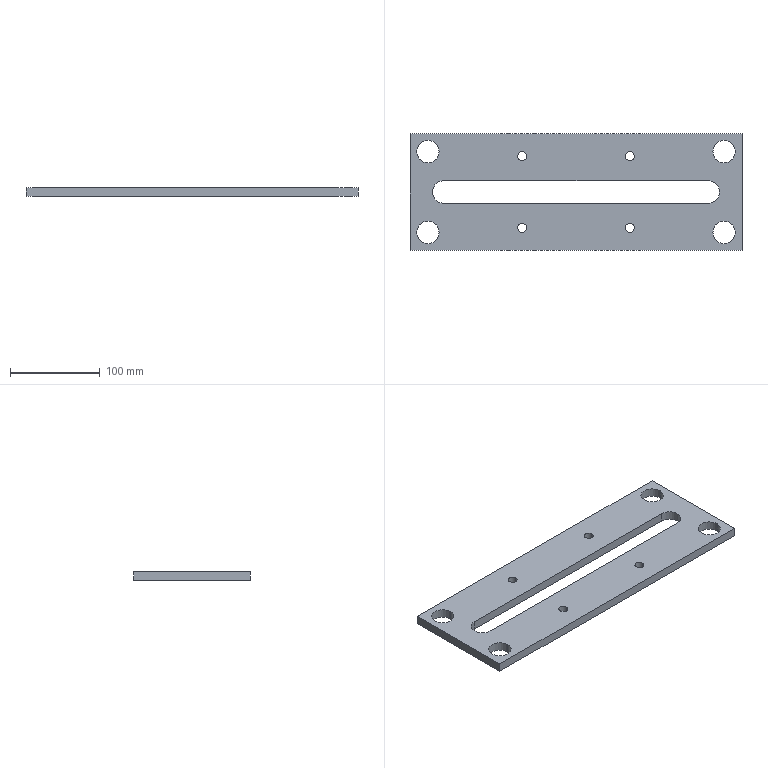Part | SolidWorks | features Extrusion 1, HoleWzd 1 | 1 solid | 27 faces | box 370 x 130 x 10 mm | volume 379565 mm3 | cylinder 19 | plane 8 | commonest cylinder face diameters 25 x11 10 x8
STEP:
#1=CARTESIAN_POINT('',(250.,25.,10.));
#2=VERTEX_POINT('',#1);
#3=CARTESIAN_POINT('',(240.,25.,10.));
#4=VERTEX_POINT('',#3);
#5=CARTESIAN_POINT('',(245.,25.,10.));
#6=DIRECTION('',(0.,0.,-1.));
#7=DIRECTION('',(-1.,0.,0.));
#8=AXIS2_PLACEMENT_3D('',#5,#6,#7);
#9=CIRCLE('',#8,5.);
#10=EDGE_CURVE('',#2,#4,#9,.T.);
#11=ORIENTED_EDGE('',*,*,#10,.F.);
#12=CARTESIAN_POINT('',(250.,25.,0.));
#13=VERTEX_POINT('',#12);
#14=CARTESIAN_POINT('',(250.,25.,0.));
#15=DIRECTION('',(0.,0.,-1.));
#16=VECTOR('',#15,1000.);
#17=LINE('',#14,#16);
#18=EDGE_CURVE('',#2,#13,#17,.T.);
#19=ORIENTED_EDGE('',*,*,#18,.T.);
#20=CARTESIAN_POINT('',(240.,25.,0.));
#21=VERTEX_POINT('',#20);
#22=CARTESIAN_POINT('',(245.,25.,0.));
#23=DIRECTION('',(0.,0.,-1.));
#24=DIRECTION('',(-1.,0.,0.));
#25=AXIS2_PLACEMENT_3D('',#22,#23,#24);
#26=CIRCLE('',#25,5.);
#27=EDGE_CURVE('',#13,#21,#26,.T.);
#28=ORIENTED_EDGE('',*,*,#27,.T.);
#29=CARTESIAN_POINT('',(240.,25.,0.));
#30=DIRECTION('',(0.,0.,-1.));
#31=VECTOR('',#30,1000.);
#32=LINE('',#29,#31);
#33=EDGE_CURVE('',#4,#21,#32,.T.);
#34=ORIENTED_EDGE('',*,*,#33,.F.);
#35=EDGE_LOOP('',(#11,#19,#28,#34));
#36=FACE_OUTER_BOUND('',#35,.T.);
#37=CARTESIAN_POINT('',(245.,25.,0.));
#38=DIRECTION('',(0.,0.,-1.));
#39=DIRECTION('',(-1.,0.,0.));
#40=AXIS2_PLACEMENT_3D('',#37,#38,#39);
#41=CYLINDRICAL_SURFACE('',#40,5.);
#42=ADVANCED_FACE('',(#36),#41,.F.);
#43=CARTESIAN_POINT('',(130.,25.,10.));
#44=VERTEX_POINT('',#43);
#45=CARTESIAN_POINT('',(120.,25.,10.));
#46=VERTEX_POINT('',#45);
#47=CARTESIAN_POINT('',(125.,25.,10.));
#48=DIRECTION('',(0.,0.,-1.));
#49=DIRECTION('',(-1.,0.,0.));
#50=AXIS2_PLACEMENT_3D('',#47,#48,#49);
#51=CIRCLE('',#50,5.);
#52=EDGE_CURVE('',#44,#46,#51,.T.);
#53=ORIENTED_EDGE('',*,*,#52,.F.);
#54=CARTESIAN_POINT('',(130.,25.,0.));
#55=VERTEX_POINT('',#54);
#56=CARTESIAN_POINT('',(130.,25.,0.));
#57=DIRECTION('',(0.,0.,-1.));
#58=VECTOR('',#57,1000.);
#59=LINE('',#56,#58);
#60=EDGE_CURVE('',#44,#55,#59,.T.);
#61=ORIENTED_EDGE('',*,*,#60,.T.);
#62=CARTESIAN_POINT('',(120.,25.,0.));
#63=VERTEX_POINT('',#62);
#64=CARTESIAN_POINT('',(125.,25.,0.));
#65=DIRECTION('',(0.,0.,-1.));
#66=DIRECTION('',(-1.,0.,0.));
#67=AXIS2_PLACEMENT_3D('',#64,#65,#66);
#68=CIRCLE('',#67,5.);
#69=EDGE_CURVE('',#55,#63,#68,.T.);
#70=ORIENTED_EDGE('',*,*,#69,.T.);
#71=CARTESIAN_POINT('',(120.,25.,0.));
#72=DIRECTION('',(0.,0.,-1.));
#73=VECTOR('',#72,1000.);
#74=LINE('',#71,#73);
#75=EDGE_CURVE('',#46,#63,#74,.T.);
#76=ORIENTED_EDGE('',*,*,#75,.F.);
#77=EDGE_LOOP('',(#53,#61,#70,#76));
#78=FACE_OUTER_BOUND('',#77,.T.);
#79=CARTESIAN_POINT('',(125.,25.,0.));
#80=DIRECTION('',(0.,0.,-1.));
#81=DIRECTION('',(-1.,0.,0.));
#82=AXIS2_PLACEMENT_3D('',#79,#80,#81);
#83=CYLINDRICAL_SURFACE('',#82,5.);
#84=ADVANCED_FACE('',(#78),#83,.F.);
#85=CARTESIAN_POINT('',(130.,105.,10.));
#86=VERTEX_POINT('',#85);
#87=CARTESIAN_POINT('',(120.,105.,10.));
#88=VERTEX_POINT('',#87);
#89=CARTESIAN_POINT('',(125.,105.,10.));
#90=DIRECTION('',(0.,0.,-1.));
#91=DIRECTION('',(-1.,0.,0.));
#92=AXIS2_PLACEMENT_3D('',#89,#90,#91);
#93=CIRCLE('',#92,5.);
#94=EDGE_CURVE('',#86,#88,#93,.T.);
#95=ORIENTED_EDGE('',*,*,#94,.F.);
#96=CARTESIAN_POINT('',(130.,105.,0.));
#97=VERTEX_POINT('',#96);
#98=CARTESIAN_POINT('',(130.,105.,0.));
#99=DIRECTION('',(0.,0.,-1.));
#100=VECTOR('',#99,1000.);
#101=LINE('',#98,#100);
#102=EDGE_CURVE('',#86,#97,#101,.T.);
#103=ORIENTED_EDGE('',*,*,#102,.T.);
#104=CARTESIAN_POINT('',(120.,105.,0.));
#105=VERTEX_POINT('',#104);
#106=CARTESIAN_POINT('',(125.,105.,0.));
#107=DIRECTION('',(0.,0.,-1.));
#108=DIRECTION('',(-1.,0.,0.));
#109=AXIS2_PLACEMENT_3D('',#106,#107,#108);
#110=CIRCLE('',#109,5.);
#111=EDGE_CURVE('',#97,#105,#110,.T.);
#112=ORIENTED_EDGE('',*,*,#111,.T.);
#113=CARTESIAN_POINT('',(120.,105.,0.));
#114=DIRECTION('',(0.,0.,-1.));
#115=VECTOR('',#114,1000.);
#116=LINE('',#113,#115);
#117=EDGE_CURVE('',#88,#105,#116,.T.);
#118=ORIENTED_EDGE('',*,*,#117,.F.);
#119=EDGE_LOOP('',(#95,#103,#112,#118));
#120=FACE_OUTER_BOUND('',#119,.T.);
#121=CARTESIAN_POINT('',(125.,105.,0.));
#122=DIRECTION('',(0.,0.,-1.));
#123=DIRECTION('',(-1.,0.,0.));
#124=AXIS2_PLACEMENT_3D('',#121,#122,#123);
#125=CYLINDRICAL_SURFACE('',#124,5.);
#126=ADVANCED_FACE('',(#120),#125,.F.);
#127=CARTESIAN_POINT('',(250.,105.,10.));
#128=VERTEX_POINT('',#127);
#129=CARTESIAN_POINT('',(240.,105.,10.));
#130=VERTEX_POINT('',#129);
#131=CARTESIAN_POINT('',(245.,105.,10.));
#132=DIRECTION('',(0.,0.,-1.));
#133=DIRECTION('',(-1.,0.,0.));
#134=AXIS2_PLACEMENT_3D('',#131,#132,#133);
#135=CIRCLE('',#134,5.);
#136=EDGE_CURVE('',#128,#130,#135,.T.);
#137=ORIENTED_EDGE('',*,*,#136,.F.);
#138=CARTESIAN_POINT('',(250.,105.,0.));
#139=VERTEX_POINT('',#138);
#140=CARTESIAN_POINT('',(250.,105.,0.));
#141=DIRECTION('',(0.,0.,-1.));
#142=VECTOR('',#141,1000.);
#143=LINE('',#140,#142);
#144=EDGE_CURVE('',#128,#139,#143,.T.);
#145=ORIENTED_EDGE('',*,*,#144,.T.);
#146=CARTESIAN_POINT('',(240.,105.,0.));
#147=VERTEX_POINT('',#146);
#148=CARTESIAN_POINT('',(245.,105.,0.));
#149=DIRECTION('',(0.,0.,-1.));
#150=DIRECTION('',(-1.,0.,0.));
#151=AXIS2_PLACEMENT_3D('',#148,#149,#150);
#152=CIRCLE('',#151,5.);
#153=EDGE_CURVE('',#139,#147,#152,.T.);
#154=ORIENTED_EDGE('',*,*,#153,.T.);
#155=CARTESIAN_POINT('',(240.,105.,0.));
#156=DIRECTION('',(0.,0.,-1.));
#157=VECTOR('',#156,1000.);
#158=LINE('',#155,#157);
#159=EDGE_CURVE('',#130,#147,#158,.T.);
#160=ORIENTED_EDGE('',*,*,#159,.F.);
#161=EDGE_LOOP('',(#137,#145,#154,#160));
#162=FACE_OUTER_BOUND('',#161,.T.);
#163=CARTESIAN_POINT('',(245.,105.,0.));
#164=DIRECTION('',(0.,0.,-1.));
#165=DIRECTION('',(-1.,0.,0.));
#166=AXIS2_PLACEMENT_3D('',#163,#164,#165);
#167=CYLINDRICAL_SURFACE('',#166,5.);
#168=ADVANCED_FACE('',(#162),#167,.F.);
#169=CARTESIAN_POINT('',(32.5,20.,10.));
#170=VERTEX_POINT('',#169);
#171=CARTESIAN_POINT('',(7.5,20.,10.));
#172=VERTEX_POINT('',#171);
#173=CARTESIAN_POINT('',(20.,20.,10.));
#174=DIRECTION('',(0.,0.,-1.));
#175=DIRECTION('',(1.,0.,0.));
#176=AXIS2_PLACEMENT_3D('',#173,#174,#175);
#177=CIRCLE('',#176,12.5);
#178=EDGE_CURVE('',#170,#172,#177,.T.);
#179=ORIENTED_EDGE('',*,*,#178,.F.);
#180=CARTESIAN_POINT('',(32.5,20.,0.));
#181=VERTEX_POINT('',#180);
#182=CARTESIAN_POINT('',(32.5,20.,10.));
#183=DIRECTION('',(0.,0.,-1.));
#184=VECTOR('',#183,1000.);
#185=LINE('',#182,#184);
#186=EDGE_CURVE('',#170,#181,#185,.T.);
#187=ORIENTED_EDGE('',*,*,#186,.T.);
#188=CARTESIAN_POINT('',(7.5,20.,0.));
#189=VERTEX_POINT('',#188);
#190=CARTESIAN_POINT('',(20.,20.,0.));
#191=DIRECTION('',(0.,0.,-1.));
#192=DIRECTION('',(1.,0.,0.));
#193=AXIS2_PLACEMENT_3D('',#190,#191,#192);
#194=CIRCLE('',#193,12.5);
#195=EDGE_CURVE('',#181,#189,#194,.T.);
#196=ORIENTED_EDGE('',*,*,#195,.T.);
#197=CARTESIAN_POINT('',(7.5,20.,10.));
#198=DIRECTION('',(0.,0.,-1.));
#199=VECTOR('',#198,1000.);
#200=LINE('',#197,#199);
#201=EDGE_CURVE('',#172,#189,#200,.T.);
#202=ORIENTED_EDGE('',*,*,#201,.F.);
#203=EDGE_LOOP('',(#179,#187,#196,#202));
#204=FACE_OUTER_BOUND('',#203,.T.);
#205=CARTESIAN_POINT('',(20.,20.,10.));
#206=DIRECTION('',(0.,0.,-1.));
#207=DIRECTION('',(-1.,0.,0.));
#208=AXIS2_PLACEMENT_3D('',#205,#206,#207);
#209=CYLINDRICAL_SURFACE('',#208,12.5);
#210=ADVANCED_FACE('',(#204),#209,.F.);
#211=CARTESIAN_POINT('',(362.5,110.,10.));
#212=VERTEX_POINT('',#211);
#213=CARTESIAN_POINT('',(337.5,110.,10.));
#214=VERTEX_POINT('',#213);
#215=CARTESIAN_POINT('',(350.,110.,10.));
#216=DIRECTION('',(0.,0.,-1.));
#217=DIRECTION('',(1.,0.,0.));
#218=AXIS2_PLACEMENT_3D('',#215,#216,#217);
#219=CIRCLE('',#218,12.5);
#220=EDGE_CURVE('',#212,#214,#219,.T.);
#221=ORIENTED_EDGE('',*,*,#220,.F.);
#222=CARTESIAN_POINT('',(362.5,110.,0.));
#223=VERTEX_POINT('',#222);
#224=CARTESIAN_POINT('',(362.5,110.,10.));
#225=DIRECTION('',(0.,0.,-1.));
#226=VECTOR('',#225,1000.);
#227=LINE('',#224,#226);
#228=EDGE_CURVE('',#212,#223,#227,.T.);
#229=ORIENTED_EDGE('',*,*,#228,.T.);
#230=CARTESIAN_POINT('',(337.5,110.,0.));
#231=VERTEX_POINT('',#230);
#232=CARTESIAN_POINT('',(350.,110.,0.));
#233=DIRECTION('',(0.,0.,-1.));
#234=DIRECTION('',(1.,0.,0.));
#235=AXIS2_PLACEMENT_3D('',#232,#233,#234);
#236=CIRCLE('',#235,12.5);
#237=EDGE_CURVE('',#223,#231,#236,.T.);
#238=ORIENTED_EDGE('',*,*,#237,.T.);
#239=CARTESIAN_POINT('',(337.5,110.,10.));
#240=DIRECTION('',(0.,0.,-1.));
#241=VECTOR('',#240,1000.);
#242=LINE('',#239,#241);
#243=EDGE_CURVE('',#214,#231,#242,.T.);
#244=ORIENTED_EDGE('',*,*,#243,.F.);
#245=EDGE_LOOP('',(#221,#229,#238,#244));
#246=FACE_OUTER_BOUND('',#245,.T.);
#247=CARTESIAN_POINT('',(350.,110.,10.));
#248=DIRECTION('',(0.,0.,-1.));
#249=DIRECTION('',(-1.,0.,0.));
#250=AXIS2_PLACEMENT_3D('',#247,#248,#249);
#251=CYLINDRICAL_SURFACE('',#250,12.5);
#252=ADVANCED_FACE('',(#246),#251,.F.);
#253=CARTESIAN_POINT('',(25.,65.,10.));
#254=VERTEX_POINT('',#253);
#255=CARTESIAN_POINT('',(37.5,77.5,10.));
#256=VERTEX_POINT('',#255);
#257=CARTESIAN_POINT('',(37.5,65.,10.));
#258=DIRECTION('',(0.,0.,-1.));
#259=DIRECTION('',(1.,0.,0.));
#260=AXIS2_PLACEMENT_3D('',#257,#258,#259);
#261=CIRCLE('',#260,12.5);
#262=EDGE_CURVE('',#254,#256,#261,.T.);
#263=ORIENTED_EDGE('',*,*,#262,.F.);
#264=CARTESIAN_POINT('',(25.,65.,0.));
#265=VERTEX_POINT('',#264);
#266=CARTESIAN_POINT('',(25.,65.,10.));
#267=DIRECTION('',(0.,0.,-1.));
#268=VECTOR('',#267,1000.);
#269=LINE('',#266,#268);
#270=EDGE_CURVE('',#254,#265,#269,.T.);
#271=ORIENTED_EDGE('',*,*,#270,.T.);
#272=CARTESIAN_POINT('',(37.5,77.5,0.));
#273=VERTEX_POINT('',#272);
#274=CARTESIAN_POINT('',(37.5,65.,0.));
#275=DIRECTION('',(0.,0.,-1.));
#276=DIRECTION('',(1.,0.,0.));
#277=AXIS2_PLACEMENT_3D('',#274,#275,#276);
#278=CIRCLE('',#277,12.5);
#279=EDGE_CURVE('',#265,#273,#278,.T.);
#280=ORIENTED_EDGE('',*,*,#279,.T.);
#281=CARTESIAN_POINT('',(37.5,77.5,10.));
#282=DIRECTION('',(0.,0.,-1.));
#283=VECTOR('',#282,1000.);
#284=LINE('',#281,#283);
#285=EDGE_CURVE('',#256,#273,#284,.T.);
#286=ORIENTED_EDGE('',*,*,#285,.F.);
#287=EDGE_LOOP('',(#263,#271,#280,#286));
#288=FACE_OUTER_BOUND('',#287,.T.);
#289=CARTESIAN_POINT('',(37.5,65.,10.));
#290=DIRECTION('',(0.,0.,-1.));
#291=DIRECTION('',(-1.,0.,0.));
#292=AXIS2_PLACEMENT_3D('',#289,#290,#291);
#293=CYLINDRICAL_SURFACE('',#292,12.5);
#294=ADVANCED_FACE('',(#288),#293,.F.);
#295=CARTESIAN_POINT('',(32.5,110.,10.));
#296=VERTEX_POINT('',#295);
#297=CARTESIAN_POINT('',(7.5,110.,10.));
#298=VERTEX_POINT('',#297);
#299=CARTESIAN_POINT('',(20.,110.,10.));
#300=DIRECTION('',(0.,0.,-1.));
#301=DIRECTION('',(1.,0.,0.));
#302=AXIS2_PLACEMENT_3D('',#299,#300,#301);
#303=CIRCLE('',#302,12.5);
#304=EDGE_CURVE('',#296,#298,#303,.T.);
#305=ORIENTED_EDGE('',*,*,#304,.F.);
#306=CARTESIAN_POINT('',(32.5,110.,0.));
#307=VERTEX_POINT('',#306);
#308=CARTESIAN_POINT('',(32.5,110.,10.));
#309=DIRECTION('',(0.,0.,-1.));
#310=VECTOR('',#309,1000.);
#311=LINE('',#308,#310);
#312=EDGE_CURVE('',#296,#307,#311,.T.);
#313=ORIENTED_EDGE('',*,*,#312,.T.);
#314=CARTESIAN_POINT('',(7.5,110.,0.));
#315=VERTEX_POINT('',#314);
#316=CARTESIAN_POINT('',(20.,110.,0.));
#317=DIRECTION('',(0.,0.,-1.));
#318=DIRECTION('',(1.,0.,0.));
#319=AXIS2_PLACEMENT_3D('',#316,#317,#318);
#320=CIRCLE('',#319,12.5);
#321=EDGE_CURVE('',#307,#315,#320,.T.);
#322=ORIENTED_EDGE('',*,*,#321,.T.);
#323=CARTESIAN_POINT('',(7.5,110.,10.));
#324=DIRECTION('',(0.,0.,-1.));
#325=VECTOR('',#324,1000.);
#326=LINE('',#323,#325);
#327=EDGE_CURVE('',#298,#315,#326,.T.);
#328=ORIENTED_EDGE('',*,*,#327,.F.);
#329=EDGE_LOOP('',(#305,#313,#322,#328));
#330=FACE_OUTER_BOUND('',#329,.T.);
#331=CARTESIAN_POINT('',(20.,110.,10.));
#332=DIRECTION('',(0.,0.,-1.));
#333=DIRECTION('',(-1.,0.,0.));
#334=AXIS2_PLACEMENT_3D('',#331,#332,#333);
#335=CYLINDRICAL_SURFACE('',#334,12.5);
#336=ADVANCED_FACE('',(#330),#335,.F.);
#337=CARTESIAN_POINT('',(362.5,20.,10.));
#338=VERTEX_POINT('',#337);
#339=CARTESIAN_POINT('',(337.5,20.,10.));
#340=VERTEX_POINT('',#339);
#341=CARTESIAN_POINT('',(350.,20.,10.));
#342=DIRECTION('',(0.,0.,-1.));
#343=DIRECTION('',(1.,0.,0.));
#344=AXIS2_PLACEMENT_3D('',#341,#342,#343);
#345=CIRCLE('',#344,12.5);
#346=EDGE_CURVE('',#338,#340,#345,.T.);
#347=ORIENTED_EDGE('',*,*,#346,.F.);
#348=CARTESIAN_POINT('',(362.5,20.,0.));
#349=VERTEX_POINT('',#348);
#350=CARTESIAN_POINT('',(362.5,20.,10.));
#351=DIRECTION('',(0.,0.,-1.));
#352=VECTOR('',#351,1000.);
#353=LINE('',#350,#352);
#354=EDGE_CURVE('',#338,#349,#353,.T.);
#355=ORIENTED_EDGE('',*,*,#354,.T.);
#356=CARTESIAN_POINT('',(337.5,20.,0.));
#357=VERTEX_POINT('',#356);
#358=CARTESIAN_POINT('',(350.,20.,0.));
#359=DIRECTION('',(0.,0.,-1.));
#360=DIRECTION('',(1.,0.,0.));
#361=AXIS2_PLACEMENT_3D('',#358,#359,#360);
#362=CIRCLE('',#361,12.5);
#363=EDGE_CURVE('',#349,#357,#362,.T.);
#364=ORIENTED_EDGE('',*,*,#363,.T.);
#365=CARTESIAN_POINT('',(337.5,20.,10.));
#366=DIRECTION('',(0.,0.,-1.));
#367=VECTOR('',#366,1000.);
#368=LINE('',#365,#367);
#369=EDGE_CURVE('',#340,#357,#368,.T.);
#370=ORIENTED_EDGE('',*,*,#369,.F.);
#371=EDGE_LOOP('',(#347,#355,#364,#370));
#372=FACE_OUTER_BOUND('',#371,.T.);
#373=CARTESIAN_POINT('',(350.,20.,10.));
#374=DIRECTION('',(0.,0.,-1.));
#375=DIRECTION('',(-1.,0.,0.));
#376=AXIS2_PLACEMENT_3D('',#373,#374,#375);
#377=CYLINDRICAL_SURFACE('',#376,12.5);
#378=ADVANCED_FACE('',(#372),#377,.F.);
#379=CARTESIAN_POINT('',(370.,0.,0.));
#380=VERTEX_POINT('',#379);
#381=CARTESIAN_POINT('',(0.,0.,0.));
#382=VERTEX_POINT('',#381);
#383=CARTESIAN_POINT('',(370.,0.,0.));
#384=DIRECTION('',(-1.,0.,0.));
#385=VECTOR('',#384,1000.);
#386=LINE('',#383,#385);
#387=EDGE_CURVE('',#380,#382,#386,.T.);
#388=ORIENTED_EDGE('',*,*,#387,.F.);
#389=CARTESIAN_POINT('',(370.,0.,10.));
#390=VERTEX_POINT('',#389);
#391=CARTESIAN_POINT('',(370.,0.,10.));
#392=DIRECTION('',(0.,0.,-1.));
#393=VECTOR('',#392,1000.);
#394=LINE('',#391,#393);
#395=EDGE_CURVE('',#390,#380,#394,.T.);
#396=ORIENTED_EDGE('',*,*,#395,.F.);
#397=CARTESIAN_POINT('',(0.,0.,10.));
#398=VERTEX_POINT('',#397);
#399=CARTESIAN_POINT('',(370.,0.,10.));
#400=DIRECTION('',(-1.,0.,0.));
#401=VECTOR('',#400,1000.);
#402=LINE('',#399,#401);
#403=EDGE_CURVE('',#390,#398,#402,.T.);
#404=ORIENTED_EDGE('',*,*,#403,.T.);
#405=CARTESIAN_POINT('',(0.,0.,10.));
#406=DIRECTION('',(0.,0.,-1.));
#407=VECTOR('',#406,1000.);
#408=LINE('',#405,#407);
#409=EDGE_CURVE('',#398,#382,#408,.T.);
#410=ORIENTED_EDGE('',*,*,#409,.T.);
#411=EDGE_LOOP('',(#388,#396,#404,#410));
#412=FACE_OUTER_BOUND('',#411,.T.);
#413=CARTESIAN_POINT('',(370.,0.,10.));
#414=DIRECTION('',(0.,-1.,0.));
#415=DIRECTION('',(1.,0.,0.));
#416=AXIS2_PLACEMENT_3D('',#413,#414,#415);
#417=PLANE('',#416);
#418=ADVANCED_FACE('',(#412),#417,.T.);
#419=CARTESIAN_POINT('',(370.,130.,0.));
#420=VERTEX_POINT('',#419);
#421=CARTESIAN_POINT('',(370.,130.,0.));
#422=DIRECTION('',(0.,-1.,0.));
#423=VECTOR('',#422,1000.);
#424=LINE('',#421,#423);
#425=EDGE_CURVE('',#420,#380,#424,.T.);
#426=ORIENTED_EDGE('',*,*,#425,.F.);
#427=CARTESIAN_POINT('',(370.,130.,10.));
#428=VERTEX_POINT('',#427);
#429=CARTESIAN_POINT('',(370.,130.,10.));
#430=DIRECTION('',(0.,0.,-1.));
#431=VECTOR('',#430,1000.);
#432=LINE('',#429,#431);
#433=EDGE_CURVE('',#428,#420,#432,.T.);
#434=ORIENTED_EDGE('',*,*,#433,.F.);
#435=CARTESIAN_POINT('',(370.,130.,10.));
#436=DIRECTION('',(0.,-1.,0.));
#437=VECTOR('',#436,1000.);
#438=LINE('',#435,#437);
#439=EDGE_CURVE('',#428,#390,#438,.T.);
#440=ORIENTED_EDGE('',*,*,#439,.T.);
#441=ORIENTED_EDGE('',*,*,#395,.T.);
#442=EDGE_LOOP('',(#426,#434,#440,#441));
#443=FACE_OUTER_BOUND('',#442,.T.);
#444=CARTESIAN_POINT('',(370.,130.,10.));
#445=DIRECTION('',(1.,0.,0.));
#446=DIRECTION('',(0.,0.,-1.));
#447=AXIS2_PLACEMENT_3D('',#444,#445,#446);
#448=PLANE('',#447);
#449=ADVANCED_FACE('',(#443),#448,.T.);
#450=CARTESIAN_POINT('',(0.,130.,0.));
#451=VERTEX_POINT('',#450);
#452=CARTESIAN_POINT('',(0.,130.,0.));
#453=DIRECTION('',(1.,0.,0.));
#454=VECTOR('',#453,1000.);
#455=LINE('',#452,#454);
#456=EDGE_CURVE('',#451,#420,#455,.T.);
#457=ORIENTED_EDGE('',*,*,#456,.F.);
#458=CARTESIAN_POINT('',(0.,130.,10.));
#459=VERTEX_POINT('',#458);
#460=CARTESIAN_POINT('',(0.,130.,10.));
#461=DIRECTION('',(0.,0.,-1.));
#462=VECTOR('',#461,1000.);
#463=LINE('',#460,#462);
#464=EDGE_CURVE('',#459,#451,#463,.T.);
#465=ORIENTED_EDGE('',*,*,#464,.F.);
#466=CARTESIAN_POINT('',(0.,130.,10.));
#467=DIRECTION('',(1.,0.,0.));
#468=VECTOR('',#467,1000.);
#469=LINE('',#466,#468);
#470=EDGE_CURVE('',#459,#428,#469,.T.);
#471=ORIENTED_EDGE('',*,*,#470,.T.);
#472=ORIENTED_EDGE('',*,*,#433,.T.);
#473=EDGE_LOOP('',(#457,#465,#471,#472));
#474=FACE_OUTER_BOUND('',#473,.T.);
#475=CARTESIAN_POINT('',(0.,130.,10.));
#476=DIRECTION('',(0.,1.,0.));
#477=DIRECTION('',(0.,0.,1.));
#478=AXIS2_PLACEMENT_3D('',#475,#476,#477);
#479=PLANE('',#478);
#480=ADVANCED_FACE('',(#474),#479,.T.);
#481=CARTESIAN_POINT('',(0.,0.,0.));
#482=DIRECTION('',(0.,1.,0.));
#483=VECTOR('',#482,1000.);
#484=LINE('',#481,#483);
#485=EDGE_CURVE('',#382,#451,#484,.T.);
#486=ORIENTED_EDGE('',*,*,#485,.F.);
#487=ORIENTED_EDGE('',*,*,#409,.F.);
#488=CARTESIAN_POINT('',(0.,0.,10.));
#489=DIRECTION('',(0.,1.,0.));
#490=VECTOR('',#489,1000.);
#491=LINE('',#488,#490);
#492=EDGE_CURVE('',#398,#459,#491,.T.);
#493=ORIENTED_EDGE('',*,*,#492,.T.);
#494=ORIENTED_EDGE('',*,*,#464,.T.);
#495=EDGE_LOOP('',(#486,#487,#493,#494));
#496=FACE_OUTER_BOUND('',#495,.T.);
#497=CARTESIAN_POINT('',(0.,0.,10.));
#498=DIRECTION('',(-1.,0.,0.));
#499=DIRECTION('',(0.,0.,1.));
#500=AXIS2_PLACEMENT_3D('',#497,#498,#499);
#501=PLANE('',#500);
#502=ADVANCED_FACE('',(#496),#501,.T.);
#503=CARTESIAN_POINT('',(245.,25.,10.));
#504=DIRECTION('',(0.,0.,-1.));
#505=DIRECTION('',(-1.,0.,0.));
#506=AXIS2_PLACEMENT_3D('',#503,#504,#505);
#507=CIRCLE('',#506,5.);
#508=EDGE_CURVE('',#4,#2,#507,.T.);
#509=ORIENTED_EDGE('',*,*,#508,.T.);
#510=ORIENTED_EDGE('',*,*,#10,.T.);
#511=EDGE_LOOP('',(#509,#510));
#512=FACE_BOUND('',#511,.T.);
#513=CARTESIAN_POINT('',(125.,25.,10.));
#514=DIRECTION('',(0.,0.,-1.));
#515=DIRECTION('',(-1.,0.,0.));
#516=AXIS2_PLACEMENT_3D('',#513,#514,#515);
#517=CIRCLE('',#516,5.);
#518=EDGE_CURVE('',#46,#44,#517,.T.);
#519=ORIENTED_EDGE('',*,*,#518,.T.);
#520=ORIENTED_EDGE('',*,*,#52,.T.);
#521=EDGE_LOOP('',(#519,#520));
#522=FACE_BOUND('',#521,.T.);
#523=CARTESIAN_POINT('',(125.,105.,10.));
#524=DIRECTION('',(0.,0.,-1.));
#525=DIRECTION('',(-1.,0.,0.));
#526=AXIS2_PLACEMENT_3D('',#523,#524,#525);
#527=CIRCLE('',#526,5.);
#528=EDGE_CURVE('',#88,#86,#527,.T.);
#529=ORIENTED_EDGE('',*,*,#528,.T.);
#530=ORIENTED_EDGE('',*,*,#94,.T.);
#531=EDGE_LOOP('',(#529,#530));
#532=FACE_BOUND('',#531,.T.);
#533=CARTESIAN_POINT('',(245.,105.,10.));
#534=DIRECTION('',(0.,0.,-1.));
#535=DIRECTION('',(-1.,0.,0.));
#536=AXIS2_PLACEMENT_3D('',#533,#534,#535);
#537=CIRCLE('',#536,5.);
#538=EDGE_CURVE('',#130,#128,#537,.T.);
#539=ORIENTED_EDGE('',*,*,#538,.T.);
#540=ORIENTED_EDGE('',*,*,#136,.T.);
#541=EDGE_LOOP('',(#539,#540));
#542=FACE_BOUND('',#541,.T.);
#543=CARTESIAN_POINT('',(20.,20.,10.));
#544=DIRECTION('',(0.,0.,-1.));
#545=DIRECTION('',(1.,0.,0.));
#546=AXIS2_PLACEMENT_3D('',#543,#544,#545);
#547=CIRCLE('',#546,12.5);
#548=EDGE_CURVE('',#172,#170,#547,.T.);
#549=ORIENTED_EDGE('',*,*,#548,.T.);
#550=ORIENTED_EDGE('',*,*,#178,.T.);
#551=EDGE_LOOP('',(#549,#550));
#552=FACE_BOUND('',#551,.T.);
#553=CARTESIAN_POINT('',(350.,110.,10.));
#554=DIRECTION('',(0.,0.,-1.));
#555=DIRECTION('',(1.,0.,0.));
#556=AXIS2_PLACEMENT_3D('',#553,#554,#555);
#557=CIRCLE('',#556,12.5);
#558=EDGE_CURVE('',#214,#212,#557,.T.);
#559=ORIENTED_EDGE('',*,*,#558,.T.);
#560=ORIENTED_EDGE('',*,*,#220,.T.);
#561=EDGE_LOOP('',(#559,#560));
#562=FACE_BOUND('',#561,.T.);
#563=CARTESIAN_POINT('',(332.5,52.5,10.));
#564=VERTEX_POINT('',#563);
#565=CARTESIAN_POINT('',(37.5,52.5,10.));
#566=VERTEX_POINT('',#565);
#567=CARTESIAN_POINT('',(37.5,52.5,10.));
#568=DIRECTION('',(-1.,0.,0.));
#569=VECTOR('',#568,1000.);
#570=LINE('',#567,#569);
#571=EDGE_CURVE('',#564,#566,#570,.T.);
#572=ORIENTED_EDGE('',*,*,#571,.T.);
#573=CARTESIAN_POINT('',(37.5,65.,10.));
#574=DIRECTION('',(0.,0.,-1.));
#575=DIRECTION('',(1.,0.,0.));
#576=AXIS2_PLACEMENT_3D('',#573,#574,#575);
#577=CIRCLE('',#576,12.5);
#578=EDGE_CURVE('',#566,#254,#577,.T.);
#579=ORIENTED_EDGE('',*,*,#578,.T.);
#580=ORIENTED_EDGE('',*,*,#262,.T.);
#581=CARTESIAN_POINT('',(332.5,77.5,10.));
#582=VERTEX_POINT('',#581);
#583=CARTESIAN_POINT('',(332.5,77.5,10.));
#584=DIRECTION('',(1.,0.,0.));
#585=VECTOR('',#584,1000.);
#586=LINE('',#583,#585);
#587=EDGE_CURVE('',#256,#582,#586,.T.);
#588=ORIENTED_EDGE('',*,*,#587,.T.);
#589=CARTESIAN_POINT('',(332.5,65.,10.));
#590=DIRECTION('',(0.,0.,-1.));
#591=DIRECTION('',(1.,0.,0.));
#592=AXIS2_PLACEMENT_3D('',#589,#590,#591);
#593=CIRCLE('',#592,12.5);
#594=EDGE_CURVE('',#582,#564,#593,.T.);
#595=ORIENTED_EDGE('',*,*,#594,.T.);
#596=EDGE_LOOP('',(#572,#579,#580,#588,#595));
#597=FACE_BOUND('',#596,.T.);
#598=CARTESIAN_POINT('',(20.,110.,10.));
#599=DIRECTION('',(0.,0.,-1.));
#600=DIRECTION('',(1.,0.,0.));
#601=AXIS2_PLACEMENT_3D('',#598,#599,#600);
#602=CIRCLE('',#601,12.5);
#603=EDGE_CURVE('',#298,#296,#602,.T.);
#604=ORIENTED_EDGE('',*,*,#603,.T.);
#605=ORIENTED_EDGE('',*,*,#304,.T.);
#606=EDGE_LOOP('',(#604,#605));
#607=FACE_BOUND('',#606,.T.);
#608=CARTESIAN_POINT('',(350.,20.,10.));
#609=DIRECTION('',(0.,0.,-1.));
#610=DIRECTION('',(1.,0.,0.));
#611=AXIS2_PLACEMENT_3D('',#608,#609,#610);
#612=CIRCLE('',#611,12.5);
#613=EDGE_CURVE('',#340,#338,#612,.T.);
#614=ORIENTED_EDGE('',*,*,#613,.T.);
#615=ORIENTED_EDGE('',*,*,#346,.T.);
#616=EDGE_LOOP('',(#614,#615));
#617=FACE_BOUND('',#616,.T.);
#618=ORIENTED_EDGE('',*,*,#403,.F.);
#619=ORIENTED_EDGE('',*,*,#439,.F.);
#620=ORIENTED_EDGE('',*,*,#470,.F.);
#621=ORIENTED_EDGE('',*,*,#492,.F.);
#622=EDGE_LOOP('',(#618,#619,#620,#621));
#623=FACE_OUTER_BOUND('',#622,.T.);
#624=CARTESIAN_POINT('',(0.,0.,10.));
#625=DIRECTION('',(0.,0.,-1.));
#626=DIRECTION('',(-1.,0.,0.));
#627=AXIS2_PLACEMENT_3D('',#624,#625,#626);
#628=PLANE('',#627);
#629=ADVANCED_FACE('',(#512,#522,#532,#542,#552,#562,#597,#607,#617,#623),#628,.F.);
#630=CARTESIAN_POINT('',(245.,25.,0.));
#631=DIRECTION('',(0.,0.,-1.));
#632=DIRECTION('',(-1.,0.,0.));
#633=AXIS2_PLACEMENT_3D('',#630,#631,#632);
#634=CIRCLE('',#633,5.);
#635=EDGE_CURVE('',#21,#13,#634,.T.);
#636=ORIENTED_EDGE('',*,*,#635,.F.);
#637=ORIENTED_EDGE('',*,*,#27,.F.);
#638=EDGE_LOOP('',(#636,#637));
#639=FACE_BOUND('',#638,.T.);
#640=CARTESIAN_POINT('',(125.,25.,0.));
#641=DIRECTION('',(0.,0.,-1.));
#642=DIRECTION('',(-1.,0.,0.));
#643=AXIS2_PLACEMENT_3D('',#640,#641,#642);
#644=CIRCLE('',#643,5.);
#645=EDGE_CURVE('',#63,#55,#644,.T.);
#646=ORIENTED_EDGE('',*,*,#645,.F.);
#647=ORIENTED_EDGE('',*,*,#69,.F.);
#648=EDGE_LOOP('',(#646,#647));
#649=FACE_BOUND('',#648,.T.);
#650=CARTESIAN_POINT('',(125.,105.,0.));
#651=DIRECTION('',(0.,0.,-1.));
#652=DIRECTION('',(-1.,0.,0.));
#653=AXIS2_PLACEMENT_3D('',#650,#651,#652);
#654=CIRCLE('',#653,5.);
#655=EDGE_CURVE('',#105,#97,#654,.T.);
#656=ORIENTED_EDGE('',*,*,#655,.F.);
#657=ORIENTED_EDGE('',*,*,#111,.F.);
#658=EDGE_LOOP('',(#656,#657));
#659=FACE_BOUND('',#658,.T.);
#660=CARTESIAN_POINT('',(245.,105.,0.));
#661=DIRECTION('',(0.,0.,-1.));
#662=DIRECTION('',(-1.,0.,0.));
#663=AXIS2_PLACEMENT_3D('',#660,#661,#662);
#664=CIRCLE('',#663,5.);
#665=EDGE_CURVE('',#147,#139,#664,.T.);
#666=ORIENTED_EDGE('',*,*,#665,.F.);
#667=ORIENTED_EDGE('',*,*,#153,.F.);
#668=EDGE_LOOP('',(#666,#667));
#669=FACE_BOUND('',#668,.T.);
#670=CARTESIAN_POINT('',(20.,20.,0.));
#671=DIRECTION('',(0.,0.,-1.));
#672=DIRECTION('',(1.,0.,0.));
#673=AXIS2_PLACEMENT_3D('',#670,#671,#672);
#674=CIRCLE('',#673,12.5);
#675=EDGE_CURVE('',#189,#181,#674,.T.);
#676=ORIENTED_EDGE('',*,*,#675,.F.);
#677=ORIENTED_EDGE('',*,*,#195,.F.);
#678=EDGE_LOOP('',(#676,#677));
#679=FACE_BOUND('',#678,.T.);
#680=CARTESIAN_POINT('',(350.,110.,0.));
#681=DIRECTION('',(0.,0.,-1.));
#682=DIRECTION('',(1.,0.,0.));
#683=AXIS2_PLACEMENT_3D('',#680,#681,#682);
#684=CIRCLE('',#683,12.5);
#685=EDGE_CURVE('',#231,#223,#684,.T.);
#686=ORIENTED_EDGE('',*,*,#685,.F.);
#687=ORIENTED_EDGE('',*,*,#237,.F.);
#688=EDGE_LOOP('',(#686,#687));
#689=FACE_BOUND('',#688,.T.);
#690=CARTESIAN_POINT('',(37.5,52.5,0.));
#691=VERTEX_POINT('',#690);
#692=CARTESIAN_POINT('',(37.5,65.,0.));
#693=DIRECTION('',(0.,0.,-1.));
#694=DIRECTION('',(1.,0.,0.));
#695=AXIS2_PLACEMENT_3D('',#692,#693,#694);
#696=CIRCLE('',#695,12.5);
#697=EDGE_CURVE('',#691,#265,#696,.T.);
#698=ORIENTED_EDGE('',*,*,#697,.F.);
#699=CARTESIAN_POINT('',(332.5,52.5,0.));
#700=VERTEX_POINT('',#699);
#701=CARTESIAN_POINT('',(37.5,52.5,0.));
#702=DIRECTION('',(-1.,0.,0.));
#703=VECTOR('',#702,1000.);
#704=LINE('',#701,#703);
#705=EDGE_CURVE('',#700,#691,#704,.T.);
#706=ORIENTED_EDGE('',*,*,#705,.F.);
#707=CARTESIAN_POINT('',(332.5,77.5,0.));
#708=VERTEX_POINT('',#707);
#709=CARTESIAN_POINT('',(332.5,65.,0.));
#710=DIRECTION('',(0.,0.,-1.));
#711=DIRECTION('',(1.,0.,0.));
#712=AXIS2_PLACEMENT_3D('',#709,#710,#711);
#713=CIRCLE('',#712,12.5);
#714=EDGE_CURVE('',#708,#700,#713,.T.);
#715=ORIENTED_EDGE('',*,*,#714,.F.);
#716=CARTESIAN_POINT('',(332.5,77.5,0.));
#717=DIRECTION('',(1.,0.,0.));
#718=VECTOR('',#717,1000.);
#719=LINE('',#716,#718);
#720=EDGE_CURVE('',#273,#708,#719,.T.);
#721=ORIENTED_EDGE('',*,*,#720,.F.);
#722=ORIENTED_EDGE('',*,*,#279,.F.);
#723=EDGE_LOOP('',(#698,#706,#715,#721,#722));
#724=FACE_BOUND('',#723,.T.);
#725=CARTESIAN_POINT('',(20.,110.,0.));
#726=DIRECTION('',(0.,0.,-1.));
#727=DIRECTION('',(1.,0.,0.));
#728=AXIS2_PLACEMENT_3D('',#725,#726,#727);
#729=CIRCLE('',#728,12.5);
#730=EDGE_CURVE('',#315,#307,#729,.T.);
#731=ORIENTED_EDGE('',*,*,#730,.F.);
#732=ORIENTED_EDGE('',*,*,#321,.F.);
#733=EDGE_LOOP('',(#731,#732));
#734=FACE_BOUND('',#733,.T.);
#735=CARTESIAN_POINT('',(350.,20.,0.));
#736=DIRECTION('',(0.,0.,-1.));
#737=DIRECTION('',(1.,0.,0.));
#738=AXIS2_PLACEMENT_3D('',#735,#736,#737);
#739=CIRCLE('',#738,12.5);
#740=EDGE_CURVE('',#357,#349,#739,.T.);
#741=ORIENTED_EDGE('',*,*,#740,.F.);
#742=ORIENTED_EDGE('',*,*,#363,.F.);
#743=EDGE_LOOP('',(#741,#742));
#744=FACE_BOUND('',#743,.T.);
#745=ORIENTED_EDGE('',*,*,#387,.T.);
#746=ORIENTED_EDGE('',*,*,#485,.T.);
#747=ORIENTED_EDGE('',*,*,#456,.T.);
#748=ORIENTED_EDGE('',*,*,#425,.T.);
#749=EDGE_LOOP('',(#745,#746,#747,#748));
#750=FACE_OUTER_BOUND('',#749,.T.);
#751=CARTESIAN_POINT('',(0.,0.,0.));
#752=DIRECTION('',(0.,0.,-1.));
#753=DIRECTION('',(-1.,0.,0.));
#754=AXIS2_PLACEMENT_3D('',#751,#752,#753);
#755=PLANE('',#754);
#756=ADVANCED_FACE('',(#639,#649,#659,#669,#679,#689,#724,#734,#744,#750),#755,.T.);
#757=ORIENTED_EDGE('',*,*,#354,.F.);
#758=ORIENTED_EDGE('',*,*,#613,.F.);
#759=ORIENTED_EDGE('',*,*,#369,.T.);
#760=ORIENTED_EDGE('',*,*,#740,.T.);
#761=EDGE_LOOP('',(#757,#758,#759,#760));
#762=FACE_OUTER_BOUND('',#761,.T.);
#763=CARTESIAN_POINT('',(350.,20.,10.));
#764=DIRECTION('',(0.,0.,-1.));
#765=DIRECTION('',(-1.,0.,0.));
#766=AXIS2_PLACEMENT_3D('',#763,#764,#765);
#767=CYLINDRICAL_SURFACE('',#766,12.5);
#768=ADVANCED_FACE('',(#762),#767,.F.);
#769=ORIENTED_EDGE('',*,*,#312,.F.);
#770=ORIENTED_EDGE('',*,*,#603,.F.);
#771=ORIENTED_EDGE('',*,*,#327,.T.);
#772=ORIENTED_EDGE('',*,*,#730,.T.);
#773=EDGE_LOOP('',(#769,#770,#771,#772));
#774=FACE_OUTER_BOUND('',#773,.T.);
#775=CARTESIAN_POINT('',(20.,110.,10.));
#776=DIRECTION('',(0.,0.,-1.));
#777=DIRECTION('',(-1.,0.,0.));
#778=AXIS2_PLACEMENT_3D('',#775,#776,#777);
#779=CYLINDRICAL_SURFACE('',#778,12.5);
#780=ADVANCED_FACE('',(#774),#779,.F.);
#781=ORIENTED_EDGE('',*,*,#270,.F.);
#782=ORIENTED_EDGE('',*,*,#578,.F.);
#783=CARTESIAN_POINT('',(37.5,52.5,10.));
#784=DIRECTION('',(0.,0.,-1.));
#785=VECTOR('',#784,1000.);
#786=LINE('',#783,#785);
#787=EDGE_CURVE('',#566,#691,#786,.T.);
#788=ORIENTED_EDGE('',*,*,#787,.T.);
#789=ORIENTED_EDGE('',*,*,#697,.T.);
#790=EDGE_LOOP('',(#781,#782,#788,#789));
#791=FACE_OUTER_BOUND('',#790,.T.);
#792=CARTESIAN_POINT('',(37.5,65.,10.));
#793=DIRECTION('',(0.,0.,-1.));
#794=DIRECTION('',(-1.,0.,0.));
#795=AXIS2_PLACEMENT_3D('',#792,#793,#794);
#796=CYLINDRICAL_SURFACE('',#795,12.5);
#797=ADVANCED_FACE('',(#791),#796,.F.);
#798=ORIENTED_EDGE('',*,*,#705,.T.);
#799=ORIENTED_EDGE('',*,*,#787,.F.);
#800=ORIENTED_EDGE('',*,*,#571,.F.);
#801=CARTESIAN_POINT('',(332.5,52.5,10.));
#802=DIRECTION('',(0.,0.,-1.));
#803=VECTOR('',#802,1000.);
#804=LINE('',#801,#803);
#805=EDGE_CURVE('',#564,#700,#804,.T.);
#806=ORIENTED_EDGE('',*,*,#805,.T.);
#807=EDGE_LOOP('',(#798,#799,#800,#806));
#808=FACE_OUTER_BOUND('',#807,.T.);
#809=CARTESIAN_POINT('',(37.5,52.5,10.));
#810=DIRECTION('',(0.,-1.,0.));
#811=DIRECTION('',(0.,0.,-1.));
#812=AXIS2_PLACEMENT_3D('',#809,#810,#811);
#813=PLANE('',#812);
#814=ADVANCED_FACE('',(#808),#813,.F.);
#815=ORIENTED_EDGE('',*,*,#714,.T.);
#816=ORIENTED_EDGE('',*,*,#805,.F.);
#817=ORIENTED_EDGE('',*,*,#594,.F.);
#818=CARTESIAN_POINT('',(332.5,77.5,10.));
#819=DIRECTION('',(0.,0.,-1.));
#820=VECTOR('',#819,1000.);
#821=LINE('',#818,#820);
#822=EDGE_CURVE('',#582,#708,#821,.T.);
#823=ORIENTED_EDGE('',*,*,#822,.T.);
#824=EDGE_LOOP('',(#815,#816,#817,#823));
#825=FACE_OUTER_BOUND('',#824,.T.);
#826=CARTESIAN_POINT('',(332.5,65.,10.));
#827=DIRECTION('',(0.,0.,-1.));
#828=DIRECTION('',(-1.,0.,0.));
#829=AXIS2_PLACEMENT_3D('',#826,#827,#828);
#830=CYLINDRICAL_SURFACE('',#829,12.5);
#831=ADVANCED_FACE('',(#825),#830,.F.);
#832=ORIENTED_EDGE('',*,*,#720,.T.);
#833=ORIENTED_EDGE('',*,*,#822,.F.);
#834=ORIENTED_EDGE('',*,*,#587,.F.);
#835=ORIENTED_EDGE('',*,*,#285,.T.);
#836=EDGE_LOOP('',(#832,#833,#834,#835));
#837=FACE_OUTER_BOUND('',#836,.T.);
#838=CARTESIAN_POINT('',(332.5,77.5,10.));
#839=DIRECTION('',(0.,1.,0.));
#840=DIRECTION('',(0.,0.,1.));
#841=AXIS2_PLACEMENT_3D('',#838,#839,#840);
#842=PLANE('',#841);
#843=ADVANCED_FACE('',(#837),#842,.F.);
#844=ORIENTED_EDGE('',*,*,#228,.F.);
#845=ORIENTED_EDGE('',*,*,#558,.F.);
#846=ORIENTED_EDGE('',*,*,#243,.T.);
#847=ORIENTED_EDGE('',*,*,#685,.T.);
#848=EDGE_LOOP('',(#844,#845,#846,#847));
#849=FACE_OUTER_BOUND('',#848,.T.);
#850=CARTESIAN_POINT('',(350.,110.,10.));
#851=DIRECTION('',(0.,0.,-1.));
#852=DIRECTION('',(-1.,0.,0.));
#853=AXIS2_PLACEMENT_3D('',#850,#851,#852);
#854=CYLINDRICAL_SURFACE('',#853,12.5);
#855=ADVANCED_FACE('',(#849),#854,.F.);
#856=ORIENTED_EDGE('',*,*,#186,.F.);
#857=ORIENTED_EDGE('',*,*,#548,.F.);
#858=ORIENTED_EDGE('',*,*,#201,.T.);
#859=ORIENTED_EDGE('',*,*,#675,.T.);
#860=EDGE_LOOP('',(#856,#857,#858,#859));
#861=FACE_OUTER_BOUND('',#860,.T.);
#862=CARTESIAN_POINT('',(20.,20.,10.));
#863=DIRECTION('',(0.,0.,-1.));
#864=DIRECTION('',(-1.,0.,0.));
#865=AXIS2_PLACEMENT_3D('',#862,#863,#864);
#866=CYLINDRICAL_SURFACE('',#865,12.5);
#867=ADVANCED_FACE('',(#861),#866,.F.);
#868=ORIENTED_EDGE('',*,*,#144,.F.);
#869=ORIENTED_EDGE('',*,*,#538,.F.);
#870=ORIENTED_EDGE('',*,*,#159,.T.);
#871=ORIENTED_EDGE('',*,*,#665,.T.);
#872=EDGE_LOOP('',(#868,#869,#870,#871));
#873=FACE_OUTER_BOUND('',#872,.T.);
#874=CARTESIAN_POINT('',(245.,105.,0.));
#875=DIRECTION('',(0.,0.,-1.));
#876=DIRECTION('',(-1.,0.,0.));
#877=AXIS2_PLACEMENT_3D('',#874,#875,#876);
#878=CYLINDRICAL_SURFACE('',#877,5.);
#879=ADVANCED_FACE('',(#873),#878,.F.);
#880=ORIENTED_EDGE('',*,*,#102,.F.);
#881=ORIENTED_EDGE('',*,*,#528,.F.);
#882=ORIENTED_EDGE('',*,*,#117,.T.);
#883=ORIENTED_EDGE('',*,*,#655,.T.);
#884=EDGE_LOOP('',(#880,#881,#882,#883));
#885=FACE_OUTER_BOUND('',#884,.T.);
#886=CARTESIAN_POINT('',(125.,105.,0.));
#887=DIRECTION('',(0.,0.,-1.));
#888=DIRECTION('',(-1.,0.,0.));
#889=AXIS2_PLACEMENT_3D('',#886,#887,#888);
#890=CYLINDRICAL_SURFACE('',#889,5.);
#891=ADVANCED_FACE('',(#885),#890,.F.);
#892=ORIENTED_EDGE('',*,*,#60,.F.);
#893=ORIENTED_EDGE('',*,*,#518,.F.);
#894=ORIENTED_EDGE('',*,*,#75,.T.);
#895=ORIENTED_EDGE('',*,*,#645,.T.);
#896=EDGE_LOOP('',(#892,#893,#894,#895));
#897=FACE_OUTER_BOUND('',#896,.T.);
#898=CARTESIAN_POINT('',(125.,25.,0.));
#899=DIRECTION('',(0.,0.,-1.));
#900=DIRECTION('',(-1.,0.,0.));
#901=AXIS2_PLACEMENT_3D('',#898,#899,#900);
#902=CYLINDRICAL_SURFACE('',#901,5.);
#903=ADVANCED_FACE('',(#897),#902,.F.);
#904=ORIENTED_EDGE('',*,*,#18,.F.);
#905=ORIENTED_EDGE('',*,*,#508,.F.);
#906=ORIENTED_EDGE('',*,*,#33,.T.);
#907=ORIENTED_EDGE('',*,*,#635,.T.);
#908=EDGE_LOOP('',(#904,#905,#906,#907));
#909=FACE_OUTER_BOUND('',#908,.T.);
#910=CARTESIAN_POINT('',(245.,25.,0.));
#911=DIRECTION('',(0.,0.,-1.));
#912=DIRECTION('',(-1.,0.,0.));
#913=AXIS2_PLACEMENT_3D('',#910,#911,#912);
#914=CYLINDRICAL_SURFACE('',#913,5.);
#915=ADVANCED_FACE('',(#909),#914,.F.);
#916=CLOSED_SHELL('',(#42,#84,#126,#168,#210,#252,#294,#336,#378,#418,#449,#480,#502,#629,#756,#768,#780,#797,#814,#831,#843,#855,#867,#879,#891,#903,#915));
#917=MANIFOLD_SOLID_BREP('',#916);
#918=CARTESIAN_POINT('',(0.,0.,0.));
#919=DIRECTION('',(0.,0.,1.));
#920=DIRECTION('',(1.,0.,0.));
#921=AXIS2_PLACEMENT_3D('',#918,#919,#920);
#922=(LENGTH_UNIT()NAMED_UNIT(*)SI_UNIT(.MILLI.,.METRE.));
#923=UNCERTAINTY_MEASURE_WITH_UNIT(LENGTH_MEASURE(0.00001),#922,'','');
#924=(NAMED_UNIT(*)PLANE_ANGLE_UNIT()SI_UNIT($,.RADIAN.));
#925=(NAMED_UNIT(*)SI_UNIT($,.STERADIAN.)SOLID_ANGLE_UNIT());
#926=(GEOMETRIC_REPRESENTATION_CONTEXT(3)GLOBAL_UNCERTAINTY_ASSIGNED_CONTEXT((#923))GLOBAL_UNIT_ASSIGNED_CONTEXT((#922,#924,#925))REPRESENTATION_CONTEXT('',''));
#927=ADVANCED_BREP_SHAPE_REPRESENTATION('',(#917,#921),#926);